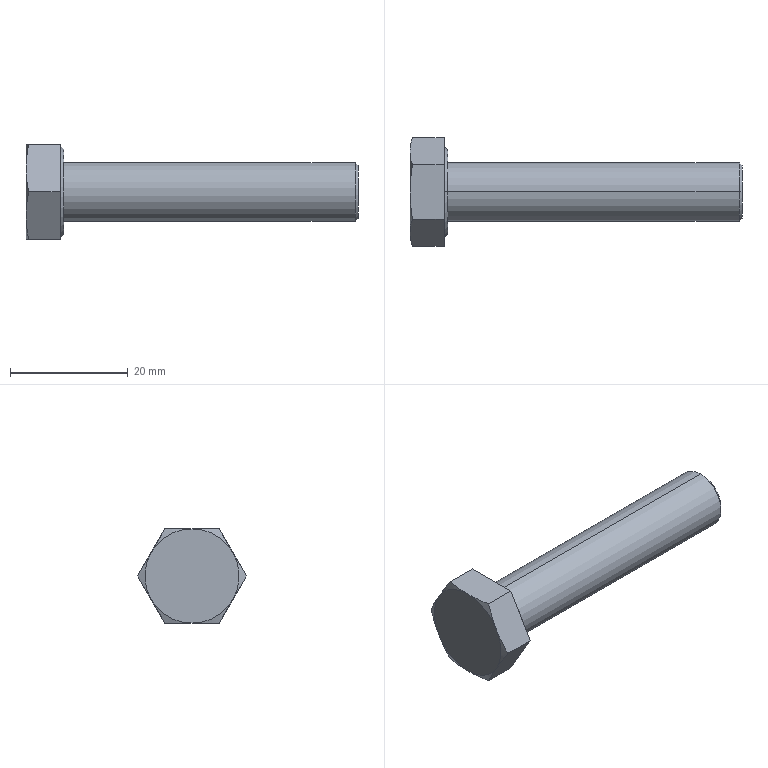Part | SolidWorks | features RevCut 3, Boss 1, Chamfer 1, Extrusion 1, Fillet 1, LPattern 1 | 1 solid | 22 faces | box 56.4 x 18.475 x 16 mm | volume 5313 mm3 | cone 10 | plane 10 | cylinder 2 | commonest cylinder face diameters 10 x2
STEP:
#1=CARTESIAN_POINT('',(56.4,0.,-4.5));
#2=VERTEX_POINT('',#1);
#3=CARTESIAN_POINT('',(56.4,0.,4.5));
#4=VERTEX_POINT('',#3);
#5=CARTESIAN_POINT('',(56.4,0.,0.));
#6=DIRECTION('',(1.,0.,0.));
#7=DIRECTION('',(0.,0.,-1.));
#8=AXIS2_PLACEMENT_3D('',#5,#6,#7);
#9=CIRCLE('',#8,4.5);
#10=EDGE_CURVE('',#2,#4,#9,.T.);
#11=ORIENTED_EDGE('',*,*,#10,.F.);
#12=CARTESIAN_POINT('',(55.9,0.,-5.));
#13=VERTEX_POINT('',#12);
#14=CARTESIAN_POINT('',(56.4,0.,-4.5));
#15=DIRECTION('',(-0.7071,0.,-0.7071));
#16=VECTOR('',#15,1000.);
#17=LINE('',#14,#16);
#18=EDGE_CURVE('',#2,#13,#17,.T.);
#19=ORIENTED_EDGE('',*,*,#18,.T.);
#20=CARTESIAN_POINT('',(55.9,0.,5.));
#21=VERTEX_POINT('',#20);
#22=CARTESIAN_POINT('',(55.9,0.,0.));
#23=DIRECTION('',(-1.,0.,0.));
#24=DIRECTION('',(0.,0.,-1.));
#25=AXIS2_PLACEMENT_3D('',#22,#23,#24);
#26=CIRCLE('',#25,5.);
#27=EDGE_CURVE('',#21,#13,#26,.T.);
#28=ORIENTED_EDGE('',*,*,#27,.F.);
#29=CARTESIAN_POINT('',(56.4,0.,4.5));
#30=DIRECTION('',(-0.7071,0.,0.7071));
#31=VECTOR('',#30,1000.);
#32=LINE('',#29,#31);
#33=EDGE_CURVE('',#4,#21,#32,.T.);
#34=ORIENTED_EDGE('',*,*,#33,.F.);
#35=EDGE_LOOP('',(#11,#19,#28,#34));
#36=FACE_OUTER_BOUND('',#35,.T.);
#37=CARTESIAN_POINT('',(56.4,0.,0.));
#38=DIRECTION('',(-1.,0.,0.));
#39=DIRECTION('',(0.,0.,1.));
#40=AXIS2_PLACEMENT_3D('',#37,#38,#39);
#41=CONICAL_SURFACE('',#40,4.5,0.7854);
#42=ADVANCED_FACE('',(#36),#41,.T.);
#43=ORIENTED_EDGE('',*,*,#27,.T.);
#44=CARTESIAN_POINT('',(6.4,0.,-5.));
#45=VERTEX_POINT('',#44);
#46=CARTESIAN_POINT('',(56.4,0.,-5.));
#47=DIRECTION('',(-1.,0.,0.));
#48=VECTOR('',#47,1000.);
#49=LINE('',#46,#48);
#50=EDGE_CURVE('',#13,#45,#49,.T.);
#51=ORIENTED_EDGE('',*,*,#50,.T.);
#52=CARTESIAN_POINT('',(6.4,0.,5.));
#53=VERTEX_POINT('',#52);
#54=CARTESIAN_POINT('',(6.4,0.,0.));
#55=DIRECTION('',(1.,0.,0.));
#56=DIRECTION('',(0.,0.,-1.));
#57=AXIS2_PLACEMENT_3D('',#54,#55,#56);
#58=CIRCLE('',#57,5.);
#59=EDGE_CURVE('',#45,#53,#58,.T.);
#60=ORIENTED_EDGE('',*,*,#59,.T.);
#61=CARTESIAN_POINT('',(56.4,0.,5.));
#62=DIRECTION('',(-1.,0.,0.));
#63=VECTOR('',#62,1000.);
#64=LINE('',#61,#63);
#65=EDGE_CURVE('',#21,#53,#64,.T.);
#66=ORIENTED_EDGE('',*,*,#65,.F.);
#67=EDGE_LOOP('',(#43,#51,#60,#66));
#68=FACE_OUTER_BOUND('',#67,.T.);
#69=CARTESIAN_POINT('',(56.4,0.,0.));
#70=DIRECTION('',(-1.,0.,0.));
#71=DIRECTION('',(0.,0.,1.));
#72=AXIS2_PLACEMENT_3D('',#69,#70,#71);
#73=CYLINDRICAL_SURFACE('',#72,5.);
#74=ADVANCED_FACE('',(#68),#73,.T.);
#75=CARTESIAN_POINT('',(6.4,0.,7.235));
#76=VERTEX_POINT('',#75);
#77=CARTESIAN_POINT('',(6.4,0.,-7.235));
#78=VERTEX_POINT('',#77);
#79=CARTESIAN_POINT('',(6.4,0.,0.));
#80=DIRECTION('',(-1.,0.,0.));
#81=DIRECTION('',(0.,0.,1.));
#82=AXIS2_PLACEMENT_3D('',#79,#80,#81);
#83=CIRCLE('',#82,7.235);
#84=EDGE_CURVE('',#76,#78,#83,.T.);
#85=ORIENTED_EDGE('',*,*,#84,.T.);
#86=CARTESIAN_POINT('',(5.8,0.,-7.835));
#87=VERTEX_POINT('',#86);
#88=CARTESIAN_POINT('',(5.8,0.,-7.835));
#89=DIRECTION('',(-0.7071,0.,-0.7071));
#90=VECTOR('',#89,1000.);
#91=LINE('',#88,#90);
#92=EDGE_CURVE('',#78,#87,#91,.T.);
#93=ORIENTED_EDGE('',*,*,#92,.T.);
#94=CARTESIAN_POINT('',(5.8,0.,7.835));
#95=VERTEX_POINT('',#94);
#96=CARTESIAN_POINT('',(5.8,0.,0.));
#97=DIRECTION('',(-1.,0.,0.));
#98=DIRECTION('',(0.,0.,1.));
#99=AXIS2_PLACEMENT_3D('',#96,#97,#98);
#100=CIRCLE('',#99,7.835);
#101=EDGE_CURVE('',#95,#87,#100,.T.);
#102=ORIENTED_EDGE('',*,*,#101,.F.);
#103=CARTESIAN_POINT('',(5.8,0.,7.835));
#104=DIRECTION('',(-0.7071,0.,0.7071));
#105=VECTOR('',#104,1000.);
#106=LINE('',#103,#105);
#107=EDGE_CURVE('',#76,#95,#106,.T.);
#108=ORIENTED_EDGE('',*,*,#107,.F.);
#109=EDGE_LOOP('',(#85,#93,#102,#108));
#110=FACE_OUTER_BOUND('',#109,.T.);
#111=CARTESIAN_POINT('',(5.8,0.,0.));
#112=DIRECTION('',(-1.,0.,0.));
#113=DIRECTION('',(0.,0.,1.));
#114=AXIS2_PLACEMENT_3D('',#111,#112,#113);
#115=CONICAL_SURFACE('',#114,7.835,0.7854);
#116=ADVANCED_FACE('',(#110),#115,.T.);
#117=ORIENTED_EDGE('',*,*,#84,.F.);
#118=CARTESIAN_POINT('',(6.4,0.,0.));
#119=DIRECTION('',(-1.,0.,0.));
#120=DIRECTION('',(0.,0.,1.));
#121=AXIS2_PLACEMENT_3D('',#118,#119,#120);
#122=CIRCLE('',#121,7.235);
#123=EDGE_CURVE('',#78,#76,#122,.T.);
#124=ORIENTED_EDGE('',*,*,#123,.F.);
#125=EDGE_LOOP('',(#117,#124));
#126=FACE_OUTER_BOUND('',#125,.T.);
#127=CARTESIAN_POINT('',(6.4,0.,0.));
#128=DIRECTION('',(1.,0.,0.));
#129=DIRECTION('',(0.,0.,-1.));
#130=AXIS2_PLACEMENT_3D('',#127,#128,#129);
#131=CIRCLE('',#130,5.);
#132=EDGE_CURVE('',#53,#45,#131,.T.);
#133=ORIENTED_EDGE('',*,*,#132,.F.);
#134=ORIENTED_EDGE('',*,*,#59,.F.);
#135=EDGE_LOOP('',(#133,#134));
#136=FACE_BOUND('',#135,.T.);
#137=CARTESIAN_POINT('',(6.4,-13.856,-8.));
#138=DIRECTION('',(1.,0.,0.));
#139=DIRECTION('',(0.,0.,-1.));
#140=AXIS2_PLACEMENT_3D('',#137,#138,#139);
#141=PLANE('',#140);
#142=ADVANCED_FACE('',(#126,#136),#141,.T.);
#143=CARTESIAN_POINT('',(0.4505,-9.238,0.));
#144=VERTEX_POINT('',#143);
#145=CARTESIAN_POINT('',(0.,-6.928,4.));
#146=VERTEX_POINT('',#145);
#147=CARTESIAN_POINT('',(0.4505,-9.238,0.));
#148=CARTESIAN_POINT('',(0.3104,-8.853,0.6667));
#149=CARTESIAN_POINT('',(0.1966,-8.468,1.333));
#150=CARTESIAN_POINT('',(0.04119,-7.698,2.667));
#151=CARTESIAN_POINT('',(0.,-7.313,3.333));
#152=CARTESIAN_POINT('',(0.,-6.928,4.));
#153=B_SPLINE_CURVE_WITH_KNOTS('',3,(#147,#148,#149,#150,#151,#152),.UNSPECIFIED.,.F.,.F.,(4,2,4),(0.000000231,0.00231,0.004619),.UNSPECIFIED.);
#154=EDGE_CURVE('',#144,#146,#153,.T.);
#155=ORIENTED_EDGE('',*,*,#154,.F.);
#156=CARTESIAN_POINT('',(5.8,-9.238,0.));
#157=VERTEX_POINT('',#156);
#158=CARTESIAN_POINT('',(6.4,-9.238,0.));
#159=DIRECTION('',(-1.,0.,0.));
#160=VECTOR('',#159,1000.);
#161=LINE('',#158,#160);
#162=EDGE_CURVE('',#157,#144,#161,.T.);
#163=ORIENTED_EDGE('',*,*,#162,.F.);
#164=CARTESIAN_POINT('',(5.8,-4.619,8.));
#165=VERTEX_POINT('',#164);
#166=CARTESIAN_POINT('',(5.8,-4.619,8.));
#167=DIRECTION('',(0.,-0.5,-0.866));
#168=VECTOR('',#167,1000.);
#169=LINE('',#166,#168);
#170=EDGE_CURVE('',#165,#157,#169,.T.);
#171=ORIENTED_EDGE('',*,*,#170,.F.);
#172=CARTESIAN_POINT('',(0.4505,-4.619,8.));
#173=VERTEX_POINT('',#172);
#174=CARTESIAN_POINT('',(6.4,-4.619,8.));
#175=DIRECTION('',(-1.,0.,0.));
#176=VECTOR('',#175,1000.);
#177=LINE('',#174,#176);
#178=EDGE_CURVE('',#165,#173,#177,.T.);
#179=ORIENTED_EDGE('',*,*,#178,.T.);
#180=CARTESIAN_POINT('',(0.,-6.928,4.));
#181=CARTESIAN_POINT('',(0.,-6.543,4.667));
#182=CARTESIAN_POINT('',(0.04119,-6.158,5.333));
#183=CARTESIAN_POINT('',(0.1966,-5.389,6.667));
#184=CARTESIAN_POINT('',(0.3104,-5.004,7.333));
#185=CARTESIAN_POINT('',(0.4505,-4.619,8.));
#186=B_SPLINE_CURVE_WITH_KNOTS('',3,(#180,#181,#182,#183,#184,#185),.UNSPECIFIED.,.F.,.F.,(4,2,4),(0.004619,0.006928,0.009238),.UNSPECIFIED.);
#187=EDGE_CURVE('',#146,#173,#186,.T.);
#188=ORIENTED_EDGE('',*,*,#187,.F.);
#189=EDGE_LOOP('',(#155,#163,#171,#179,#188));
#190=FACE_OUTER_BOUND('',#189,.T.);
#191=CARTESIAN_POINT('',(6.4,-4.619,8.));
#192=DIRECTION('',(0.,0.866,-0.5));
#193=DIRECTION('',(0.,0.5,0.866));
#194=AXIS2_PLACEMENT_3D('',#191,#192,#193);
#195=PLANE('',#194);
#196=ADVANCED_FACE('',(#190),#195,.F.);
#197=CARTESIAN_POINT('',(0.4505,-4.619,-8.));
#198=VERTEX_POINT('',#197);
#199=CARTESIAN_POINT('',(0.,-6.928,-4.));
#200=VERTEX_POINT('',#199);
#201=CARTESIAN_POINT('',(0.4505,-4.619,-8.));
#202=CARTESIAN_POINT('',(0.3104,-5.004,-7.333));
#203=CARTESIAN_POINT('',(0.1966,-5.389,-6.667));
#204=CARTESIAN_POINT('',(0.04119,-6.158,-5.333));
#205=CARTESIAN_POINT('',(0.,-6.543,-4.667));
#206=CARTESIAN_POINT('',(0.,-6.928,-4.));
#207=B_SPLINE_CURVE_WITH_KNOTS('',3,(#201,#202,#203,#204,#205,#206),.UNSPECIFIED.,.F.,.F.,(4,2,4),(0.000000231,0.00231,0.004619),.UNSPECIFIED.);
#208=EDGE_CURVE('',#198,#200,#207,.T.);
#209=ORIENTED_EDGE('',*,*,#208,.F.);
#210=CARTESIAN_POINT('',(5.8,-4.619,-8.));
#211=VERTEX_POINT('',#210);
#212=CARTESIAN_POINT('',(6.4,-4.619,-8.));
#213=DIRECTION('',(-1.,0.,0.));
#214=VECTOR('',#213,1000.);
#215=LINE('',#212,#214);
#216=EDGE_CURVE('',#211,#198,#215,.T.);
#217=ORIENTED_EDGE('',*,*,#216,.F.);
#218=CARTESIAN_POINT('',(5.8,-9.238,0.));
#219=DIRECTION('',(0.,0.5,-0.866));
#220=VECTOR('',#219,1000.);
#221=LINE('',#218,#220);
#222=EDGE_CURVE('',#157,#211,#221,.T.);
#223=ORIENTED_EDGE('',*,*,#222,.F.);
#224=ORIENTED_EDGE('',*,*,#162,.T.);
#225=CARTESIAN_POINT('',(0.,-6.928,-4.));
#226=CARTESIAN_POINT('',(0.,-7.313,-3.333));
#227=CARTESIAN_POINT('',(0.04119,-7.698,-2.667));
#228=CARTESIAN_POINT('',(0.1966,-8.468,-1.333));
#229=CARTESIAN_POINT('',(0.3104,-8.853,-0.6667));
#230=CARTESIAN_POINT('',(0.4505,-9.238,0.));
#231=B_SPLINE_CURVE_WITH_KNOTS('',3,(#225,#226,#227,#228,#229,#230),.UNSPECIFIED.,.F.,.F.,(4,2,4),(0.004619,0.006928,0.009238),.UNSPECIFIED.);
#232=EDGE_CURVE('',#200,#144,#231,.T.);
#233=ORIENTED_EDGE('',*,*,#232,.F.);
#234=EDGE_LOOP('',(#209,#217,#223,#224,#233));
#235=FACE_OUTER_BOUND('',#234,.T.);
#236=CARTESIAN_POINT('',(6.4,-9.238,0.));
#237=DIRECTION('',(0.,0.866,0.5));
#238=DIRECTION('',(0.,-0.5,0.866));
#239=AXIS2_PLACEMENT_3D('',#236,#237,#238);
#240=PLANE('',#239);
#241=ADVANCED_FACE('',(#235),#240,.F.);
#242=CARTESIAN_POINT('',(0.4505,4.619,-8.));
#243=VERTEX_POINT('',#242);
#244=CARTESIAN_POINT('',(0.,0.,-8.));
#245=VERTEX_POINT('',#244);
#246=CARTESIAN_POINT('',(0.4505,4.619,-8.));
#247=CARTESIAN_POINT('',(0.3107,3.851,-8.));
#248=CARTESIAN_POINT('',(0.1969,3.081,-8.));
#249=CARTESIAN_POINT('',(0.04135,1.542,-8.));
#250=CARTESIAN_POINT('',(0.,0.7714,-8.));
#251=CARTESIAN_POINT('',(0.,0.,-8.));
#252=B_SPLINE_CURVE_WITH_KNOTS('',3,(#246,#247,#248,#249,#250,#251),.UNSPECIFIED.,.F.,.F.,(4,2,4),(0.01666,0.01898,0.02131),.UNSPECIFIED.);
#253=EDGE_CURVE('',#243,#245,#252,.T.);
#254=ORIENTED_EDGE('',*,*,#253,.F.);
#255=CARTESIAN_POINT('',(5.8,4.619,-8.));
#256=VERTEX_POINT('',#255);
#257=CARTESIAN_POINT('',(6.4,4.619,-8.));
#258=DIRECTION('',(-1.,0.,0.));
#259=VECTOR('',#258,1000.);
#260=LINE('',#257,#259);
#261=EDGE_CURVE('',#256,#243,#260,.T.);
#262=ORIENTED_EDGE('',*,*,#261,.F.);
#263=CARTESIAN_POINT('',(5.8,-4.619,-8.));
#264=DIRECTION('',(0.,1.,0.));
#265=VECTOR('',#264,1000.);
#266=LINE('',#263,#265);
#267=EDGE_CURVE('',#211,#256,#266,.T.);
#268=ORIENTED_EDGE('',*,*,#267,.F.);
#269=ORIENTED_EDGE('',*,*,#216,.T.);
#270=CARTESIAN_POINT('',(0.,0.,-8.));
#271=CARTESIAN_POINT('',(0.,-0.7692,-8.));
#272=CARTESIAN_POINT('',(0.04113,-1.539,-8.));
#273=CARTESIAN_POINT('',(0.1968,-3.081,-8.));
#274=CARTESIAN_POINT('',(0.3113,-3.854,-8.));
#275=CARTESIAN_POINT('',(0.4505,-4.619,-8.));
#276=B_SPLINE_CURVE_WITH_KNOTS('',3,(#270,#271,#272,#273,#274,#275),.UNSPECIFIED.,.F.,.F.,(4,2,4),(0.02131,0.02363,0.02596),.UNSPECIFIED.);
#277=EDGE_CURVE('',#245,#198,#276,.T.);
#278=ORIENTED_EDGE('',*,*,#277,.F.);
#279=EDGE_LOOP('',(#254,#262,#268,#269,#278));
#280=FACE_OUTER_BOUND('',#279,.T.);
#281=CARTESIAN_POINT('',(6.4,-4.619,-8.));
#282=DIRECTION('',(0.,0.,1.));
#283=DIRECTION('',(1.,0.,0.));
#284=AXIS2_PLACEMENT_3D('',#281,#282,#283);
#285=PLANE('',#284);
#286=ADVANCED_FACE('',(#280),#285,.F.);
#287=CARTESIAN_POINT('',(0.4505,9.238,0.));
#288=VERTEX_POINT('',#287);
#289=CARTESIAN_POINT('',(0.,6.928,-4.));
#290=VERTEX_POINT('',#289);
#291=CARTESIAN_POINT('',(0.4505,9.238,0.));
#292=CARTESIAN_POINT('',(0.3104,8.853,-0.6667));
#293=CARTESIAN_POINT('',(0.1966,8.468,-1.333));
#294=CARTESIAN_POINT('',(0.04119,7.698,-2.667));
#295=CARTESIAN_POINT('',(0.,7.313,-3.333));
#296=CARTESIAN_POINT('',(0.,6.928,-4.));
#297=B_SPLINE_CURVE_WITH_KNOTS('',3,(#291,#292,#293,#294,#295,#296),.UNSPECIFIED.,.F.,.F.,(4,2,4),(0.000000231,0.00231,0.004619),.UNSPECIFIED.);
#298=EDGE_CURVE('',#288,#290,#297,.T.);
#299=ORIENTED_EDGE('',*,*,#298,.F.);
#300=CARTESIAN_POINT('',(5.8,9.238,0.));
#301=VERTEX_POINT('',#300);
#302=CARTESIAN_POINT('',(6.4,9.238,0.));
#303=DIRECTION('',(-1.,0.,0.));
#304=VECTOR('',#303,1000.);
#305=LINE('',#302,#304);
#306=EDGE_CURVE('',#301,#288,#305,.T.);
#307=ORIENTED_EDGE('',*,*,#306,.F.);
#308=CARTESIAN_POINT('',(5.8,4.619,-8.));
#309=DIRECTION('',(0.,0.5,0.866));
#310=VECTOR('',#309,1000.);
#311=LINE('',#308,#310);
#312=EDGE_CURVE('',#256,#301,#311,.T.);
#313=ORIENTED_EDGE('',*,*,#312,.F.);
#314=ORIENTED_EDGE('',*,*,#261,.T.);
#315=CARTESIAN_POINT('',(0.,6.928,-4.));
#316=CARTESIAN_POINT('',(0.,6.543,-4.667));
#317=CARTESIAN_POINT('',(0.04119,6.158,-5.333));
#318=CARTESIAN_POINT('',(0.1966,5.389,-6.667));
#319=CARTESIAN_POINT('',(0.3104,5.004,-7.333));
#320=CARTESIAN_POINT('',(0.4505,4.619,-8.));
#321=B_SPLINE_CURVE_WITH_KNOTS('',3,(#315,#316,#317,#318,#319,#320),.UNSPECIFIED.,.F.,.F.,(4,2,4),(0.004619,0.006928,0.009238),.UNSPECIFIED.);
#322=EDGE_CURVE('',#290,#243,#321,.T.);
#323=ORIENTED_EDGE('',*,*,#322,.F.);
#324=EDGE_LOOP('',(#299,#307,#313,#314,#323));
#325=FACE_OUTER_BOUND('',#324,.T.);
#326=CARTESIAN_POINT('',(6.4,4.619,-8.));
#327=DIRECTION('',(0.,-0.866,0.5));
#328=DIRECTION('',(0.,-0.5,-0.866));
#329=AXIS2_PLACEMENT_3D('',#326,#327,#328);
#330=PLANE('',#329);
#331=ADVANCED_FACE('',(#325),#330,.F.);
#332=CARTESIAN_POINT('',(0.4505,4.619,8.));
#333=VERTEX_POINT('',#332);
#334=CARTESIAN_POINT('',(0.,6.928,4.));
#335=VERTEX_POINT('',#334);
#336=CARTESIAN_POINT('',(0.4505,4.619,8.));
#337=CARTESIAN_POINT('',(0.3104,5.004,7.333));
#338=CARTESIAN_POINT('',(0.1966,5.389,6.667));
#339=CARTESIAN_POINT('',(0.04119,6.158,5.333));
#340=CARTESIAN_POINT('',(0.,6.543,4.667));
#341=CARTESIAN_POINT('',(0.,6.928,4.));
#342=B_SPLINE_CURVE_WITH_KNOTS('',3,(#336,#337,#338,#339,#340,#341),.UNSPECIFIED.,.F.,.F.,(4,2,4),(0.000000231,0.00231,0.004619),.UNSPECIFIED.);
#343=EDGE_CURVE('',#333,#335,#342,.T.);
#344=ORIENTED_EDGE('',*,*,#343,.F.);
#345=CARTESIAN_POINT('',(5.8,4.619,8.));
#346=VERTEX_POINT('',#345);
#347=CARTESIAN_POINT('',(6.4,4.619,8.));
#348=DIRECTION('',(-1.,0.,0.));
#349=VECTOR('',#348,1000.);
#350=LINE('',#347,#349);
#351=EDGE_CURVE('',#346,#333,#350,.T.);
#352=ORIENTED_EDGE('',*,*,#351,.F.);
#353=CARTESIAN_POINT('',(5.8,9.238,0.));
#354=DIRECTION('',(0.,-0.5,0.866));
#355=VECTOR('',#354,1000.);
#356=LINE('',#353,#355);
#357=EDGE_CURVE('',#301,#346,#356,.T.);
#358=ORIENTED_EDGE('',*,*,#357,.F.);
#359=ORIENTED_EDGE('',*,*,#306,.T.);
#360=CARTESIAN_POINT('',(0.,6.928,4.));
#361=CARTESIAN_POINT('',(0.,7.313,3.333));
#362=CARTESIAN_POINT('',(0.04119,7.698,2.667));
#363=CARTESIAN_POINT('',(0.1966,8.468,1.333));
#364=CARTESIAN_POINT('',(0.3104,8.853,0.6667));
#365=CARTESIAN_POINT('',(0.4505,9.238,0.));
#366=B_SPLINE_CURVE_WITH_KNOTS('',3,(#360,#361,#362,#363,#364,#365),.UNSPECIFIED.,.F.,.F.,(4,2,4),(0.004619,0.006928,0.009238),.UNSPECIFIED.);
#367=EDGE_CURVE('',#335,#288,#366,.T.);
#368=ORIENTED_EDGE('',*,*,#367,.F.);
#369=EDGE_LOOP('',(#344,#352,#358,#359,#368));
#370=FACE_OUTER_BOUND('',#369,.T.);
#371=CARTESIAN_POINT('',(6.4,9.238,0.));
#372=DIRECTION('',(0.,-0.866,-0.5));
#373=DIRECTION('',(0.,0.5,-0.866));
#374=AXIS2_PLACEMENT_3D('',#371,#372,#373);
#375=PLANE('',#374);
#376=ADVANCED_FACE('',(#370),#375,.F.);
#377=CARTESIAN_POINT('',(0.,0.,8.));
#378=VERTEX_POINT('',#377);
#379=CARTESIAN_POINT('',(0.4505,-4.619,8.));
#380=CARTESIAN_POINT('',(0.3113,-3.854,8.));
#381=CARTESIAN_POINT('',(0.1968,-3.081,8.));
#382=CARTESIAN_POINT('',(0.04113,-1.539,8.));
#383=CARTESIAN_POINT('',(0.,-0.7692,8.));
#384=CARTESIAN_POINT('',(0.,0.,8.));
#385=B_SPLINE_CURVE_WITH_KNOTS('',3,(#379,#380,#381,#382,#383,#384),.UNSPECIFIED.,.F.,.F.,(4,2,4),(0.007857,0.01018,0.01251),.UNSPECIFIED.);
#386=EDGE_CURVE('',#173,#378,#385,.T.);
#387=ORIENTED_EDGE('',*,*,#386,.F.);
#388=ORIENTED_EDGE('',*,*,#178,.F.);
#389=CARTESIAN_POINT('',(5.8,4.619,8.));
#390=DIRECTION('',(0.,-1.,0.));
#391=VECTOR('',#390,1000.);
#392=LINE('',#389,#391);
#393=EDGE_CURVE('',#346,#165,#392,.T.);
#394=ORIENTED_EDGE('',*,*,#393,.F.);
#395=ORIENTED_EDGE('',*,*,#351,.T.);
#396=CARTESIAN_POINT('',(0.,0.,8.));
#397=CARTESIAN_POINT('',(0.,0.7714,8.));
#398=CARTESIAN_POINT('',(0.04135,1.542,8.));
#399=CARTESIAN_POINT('',(0.1969,3.081,8.));
#400=CARTESIAN_POINT('',(0.3107,3.851,8.));
#401=CARTESIAN_POINT('',(0.4505,4.619,8.));
#402=B_SPLINE_CURVE_WITH_KNOTS('',3,(#396,#397,#398,#399,#400,#401),.UNSPECIFIED.,.F.,.F.,(4,2,4),(0.01251,0.01485,0.01718),.UNSPECIFIED.);
#403=EDGE_CURVE('',#378,#333,#402,.T.);
#404=ORIENTED_EDGE('',*,*,#403,.F.);
#405=EDGE_LOOP('',(#387,#388,#394,#395,#404));
#406=FACE_OUTER_BOUND('',#405,.T.);
#407=CARTESIAN_POINT('',(6.4,4.619,8.));
#408=DIRECTION('',(0.,0.,-1.));
#409=DIRECTION('',(0.,1.,0.));
#410=AXIS2_PLACEMENT_3D('',#407,#408,#409);
#411=PLANE('',#410);
#412=ADVANCED_FACE('',(#406),#411,.F.);
#413=ORIENTED_EDGE('',*,*,#101,.T.);
#414=CARTESIAN_POINT('',(5.8,0.,0.));
#415=DIRECTION('',(-1.,0.,0.));
#416=DIRECTION('',(0.,0.,1.));
#417=AXIS2_PLACEMENT_3D('',#414,#415,#416);
#418=CIRCLE('',#417,7.835);
#419=EDGE_CURVE('',#87,#95,#418,.T.);
#420=ORIENTED_EDGE('',*,*,#419,.T.);
#421=EDGE_LOOP('',(#413,#420));
#422=FACE_BOUND('',#421,.T.);
#423=ORIENTED_EDGE('',*,*,#170,.T.);
#424=ORIENTED_EDGE('',*,*,#222,.T.);
#425=ORIENTED_EDGE('',*,*,#267,.T.);
#426=ORIENTED_EDGE('',*,*,#312,.T.);
#427=ORIENTED_EDGE('',*,*,#357,.T.);
#428=ORIENTED_EDGE('',*,*,#393,.T.);
#429=EDGE_LOOP('',(#423,#424,#425,#426,#427,#428));
#430=FACE_OUTER_BOUND('',#429,.T.);
#431=CARTESIAN_POINT('',(5.8,7.835,0.));
#432=DIRECTION('',(1.,0.,0.));
#433=DIRECTION('',(0.,0.,-1.));
#434=AXIS2_PLACEMENT_3D('',#431,#432,#433);
#435=PLANE('',#434);
#436=ADVANCED_FACE('',(#422,#430),#435,.T.);
#437=ORIENTED_EDGE('',*,*,#92,.F.);
#438=ORIENTED_EDGE('',*,*,#123,.T.);
#439=ORIENTED_EDGE('',*,*,#107,.T.);
#440=ORIENTED_EDGE('',*,*,#419,.F.);
#441=EDGE_LOOP('',(#437,#438,#439,#440));
#442=FACE_OUTER_BOUND('',#441,.T.);
#443=CARTESIAN_POINT('',(5.8,0.,0.));
#444=DIRECTION('',(-1.,0.,0.));
#445=DIRECTION('',(0.,0.,1.));
#446=AXIS2_PLACEMENT_3D('',#443,#444,#445);
#447=CONICAL_SURFACE('',#446,7.835,0.7854);
#448=ADVANCED_FACE('',(#442),#447,.T.);
#449=ORIENTED_EDGE('',*,*,#277,.T.);
#450=ORIENTED_EDGE('',*,*,#208,.T.);
#451=CARTESIAN_POINT('',(0.,0.,0.));
#452=DIRECTION('',(1.,0.,0.));
#453=DIRECTION('',(0.,0.,-1.));
#454=AXIS2_PLACEMENT_3D('',#451,#452,#453);
#455=CIRCLE('',#454,8.);
#456=EDGE_CURVE('',#200,#245,#455,.T.);
#457=ORIENTED_EDGE('',*,*,#456,.T.);
#458=EDGE_LOOP('',(#449,#450,#457));
#459=FACE_OUTER_BOUND('',#458,.T.);
#460=CARTESIAN_POINT('',(0.,0.,0.));
#461=DIRECTION('',(1.,0.,0.));
#462=DIRECTION('',(0.,0.,-1.));
#463=AXIS2_PLACEMENT_3D('',#460,#461,#462);
#464=CONICAL_SURFACE('',#463,8.,1.222);
#465=ADVANCED_FACE('',(#459),#464,.T.);
#466=ORIENTED_EDGE('',*,*,#232,.T.);
#467=ORIENTED_EDGE('',*,*,#154,.T.);
#468=CARTESIAN_POINT('',(0.,0.,0.));
#469=DIRECTION('',(1.,0.,0.));
#470=DIRECTION('',(0.,0.,-1.));
#471=AXIS2_PLACEMENT_3D('',#468,#469,#470);
#472=CIRCLE('',#471,8.);
#473=EDGE_CURVE('',#146,#200,#472,.T.);
#474=ORIENTED_EDGE('',*,*,#473,.T.);
#475=EDGE_LOOP('',(#466,#467,#474));
#476=FACE_OUTER_BOUND('',#475,.T.);
#477=CARTESIAN_POINT('',(0.,0.,0.));
#478=DIRECTION('',(1.,0.,0.));
#479=DIRECTION('',(0.,0.,-1.));
#480=AXIS2_PLACEMENT_3D('',#477,#478,#479);
#481=CONICAL_SURFACE('',#480,8.,1.222);
#482=ADVANCED_FACE('',(#476),#481,.T.);
#483=ORIENTED_EDGE('',*,*,#187,.T.);
#484=ORIENTED_EDGE('',*,*,#386,.T.);
#485=CARTESIAN_POINT('',(0.,0.,0.));
#486=DIRECTION('',(1.,0.,0.));
#487=DIRECTION('',(0.,0.,-1.));
#488=AXIS2_PLACEMENT_3D('',#485,#486,#487);
#489=CIRCLE('',#488,8.);
#490=EDGE_CURVE('',#378,#146,#489,.T.);
#491=ORIENTED_EDGE('',*,*,#490,.T.);
#492=EDGE_LOOP('',(#483,#484,#491));
#493=FACE_OUTER_BOUND('',#492,.T.);
#494=CARTESIAN_POINT('',(0.,0.,0.));
#495=DIRECTION('',(1.,0.,0.));
#496=DIRECTION('',(0.,0.,-1.));
#497=AXIS2_PLACEMENT_3D('',#494,#495,#496);
#498=CONICAL_SURFACE('',#497,8.,1.222);
#499=ADVANCED_FACE('',(#493),#498,.T.);
#500=ORIENTED_EDGE('',*,*,#343,.T.);
#501=CARTESIAN_POINT('',(0.,0.,0.));
#502=DIRECTION('',(-1.,0.,0.));
#503=DIRECTION('',(0.,0.,1.));
#504=AXIS2_PLACEMENT_3D('',#501,#502,#503);
#505=CIRCLE('',#504,8.);
#506=EDGE_CURVE('',#378,#335,#505,.T.);
#507=ORIENTED_EDGE('',*,*,#506,.F.);
#508=ORIENTED_EDGE('',*,*,#403,.T.);
#509=EDGE_LOOP('',(#500,#507,#508));
#510=FACE_OUTER_BOUND('',#509,.T.);
#511=CARTESIAN_POINT('',(0.,0.,0.));
#512=DIRECTION('',(1.,0.,0.));
#513=DIRECTION('',(0.,0.,-1.));
#514=AXIS2_PLACEMENT_3D('',#511,#512,#513);
#515=CONICAL_SURFACE('',#514,8.,1.222);
#516=ADVANCED_FACE('',(#510),#515,.T.);
#517=ORIENTED_EDGE('',*,*,#298,.T.);
#518=CARTESIAN_POINT('',(0.,0.,0.));
#519=DIRECTION('',(1.,0.,0.));
#520=DIRECTION('',(0.,0.,-1.));
#521=AXIS2_PLACEMENT_3D('',#518,#519,#520);
#522=CIRCLE('',#521,8.);
#523=EDGE_CURVE('',#290,#335,#522,.T.);
#524=ORIENTED_EDGE('',*,*,#523,.T.);
#525=ORIENTED_EDGE('',*,*,#367,.T.);
#526=EDGE_LOOP('',(#517,#524,#525));
#527=FACE_OUTER_BOUND('',#526,.T.);
#528=CARTESIAN_POINT('',(0.,0.,0.));
#529=DIRECTION('',(1.,0.,0.));
#530=DIRECTION('',(0.,0.,-1.));
#531=AXIS2_PLACEMENT_3D('',#528,#529,#530);
#532=CONICAL_SURFACE('',#531,8.,1.222);
#533=ADVANCED_FACE('',(#527),#532,.T.);
#534=ORIENTED_EDGE('',*,*,#253,.T.);
#535=CARTESIAN_POINT('',(0.,0.,0.));
#536=DIRECTION('',(1.,0.,0.));
#537=DIRECTION('',(0.,0.,-1.));
#538=AXIS2_PLACEMENT_3D('',#535,#536,#537);
#539=CIRCLE('',#538,8.);
#540=EDGE_CURVE('',#245,#290,#539,.T.);
#541=ORIENTED_EDGE('',*,*,#540,.T.);
#542=ORIENTED_EDGE('',*,*,#322,.T.);
#543=EDGE_LOOP('',(#534,#541,#542));
#544=FACE_OUTER_BOUND('',#543,.T.);
#545=CARTESIAN_POINT('',(0.,0.,0.));
#546=DIRECTION('',(1.,0.,0.));
#547=DIRECTION('',(0.,0.,-1.));
#548=AXIS2_PLACEMENT_3D('',#545,#546,#547);
#549=CONICAL_SURFACE('',#548,8.,1.222);
#550=ADVANCED_FACE('',(#544),#549,.T.);
#551=ORIENTED_EDGE('',*,*,#540,.F.);
#552=ORIENTED_EDGE('',*,*,#456,.F.);
#553=ORIENTED_EDGE('',*,*,#473,.F.);
#554=ORIENTED_EDGE('',*,*,#490,.F.);
#555=ORIENTED_EDGE('',*,*,#506,.T.);
#556=ORIENTED_EDGE('',*,*,#523,.F.);
#557=EDGE_LOOP('',(#551,#552,#553,#554,#555,#556));
#558=FACE_OUTER_BOUND('',#557,.T.);
#559=CARTESIAN_POINT('',(0.,-13.856,-8.));
#560=DIRECTION('',(1.,0.,0.));
#561=DIRECTION('',(0.,0.,-1.));
#562=AXIS2_PLACEMENT_3D('',#559,#560,#561);
#563=PLANE('',#562);
#564=ADVANCED_FACE('',(#558),#563,.F.);
#565=ORIENTED_EDGE('',*,*,#50,.F.);
#566=CARTESIAN_POINT('',(55.9,0.,0.));
#567=DIRECTION('',(-1.,0.,0.));
#568=DIRECTION('',(0.,0.,-1.));
#569=AXIS2_PLACEMENT_3D('',#566,#567,#568);
#570=CIRCLE('',#569,5.);
#571=EDGE_CURVE('',#13,#21,#570,.T.);
#572=ORIENTED_EDGE('',*,*,#571,.T.);
#573=ORIENTED_EDGE('',*,*,#65,.T.);
#574=ORIENTED_EDGE('',*,*,#132,.T.);
#575=EDGE_LOOP('',(#565,#572,#573,#574));
#576=FACE_OUTER_BOUND('',#575,.T.);
#577=CARTESIAN_POINT('',(56.4,0.,0.));
#578=DIRECTION('',(-1.,0.,0.));
#579=DIRECTION('',(0.,0.,1.));
#580=AXIS2_PLACEMENT_3D('',#577,#578,#579);
#581=CYLINDRICAL_SURFACE('',#580,5.);
#582=ADVANCED_FACE('',(#576),#581,.T.);
#583=CARTESIAN_POINT('',(56.4,0.,0.));
#584=DIRECTION('',(1.,0.,0.));
#585=DIRECTION('',(0.,0.,-1.));
#586=AXIS2_PLACEMENT_3D('',#583,#584,#585);
#587=CIRCLE('',#586,4.5);
#588=EDGE_CURVE('',#4,#2,#587,.T.);
#589=ORIENTED_EDGE('',*,*,#588,.T.);
#590=ORIENTED_EDGE('',*,*,#10,.T.);
#591=EDGE_LOOP('',(#589,#590));
#592=FACE_OUTER_BOUND('',#591,.T.);
#593=CARTESIAN_POINT('',(56.4,0.,0.));
#594=DIRECTION('',(1.,0.,0.));
#595=DIRECTION('',(0.,0.,-1.));
#596=AXIS2_PLACEMENT_3D('',#593,#594,#595);
#597=PLANE('',#596);
#598=ADVANCED_FACE('',(#592),#597,.T.);
#599=ORIENTED_EDGE('',*,*,#18,.F.);
#600=ORIENTED_EDGE('',*,*,#588,.F.);
#601=ORIENTED_EDGE('',*,*,#33,.T.);
#602=ORIENTED_EDGE('',*,*,#571,.F.);
#603=EDGE_LOOP('',(#599,#600,#601,#602));
#604=FACE_OUTER_BOUND('',#603,.T.);
#605=CARTESIAN_POINT('',(56.4,0.,0.));
#606=DIRECTION('',(-1.,0.,0.));
#607=DIRECTION('',(0.,0.,1.));
#608=AXIS2_PLACEMENT_3D('',#605,#606,#607);
#609=CONICAL_SURFACE('',#608,4.5,0.7854);
#610=ADVANCED_FACE('',(#604),#609,.T.);
#611=CLOSED_SHELL('',(#42,#74,#116,#142,#196,#241,#286,#331,#376,#412,#436,#448,#465,#482,#499,#516,#533,#550,#564,#582,#598,#610));
#612=MANIFOLD_SOLID_BREP('',#611);
#613=CARTESIAN_POINT('',(0.,0.,0.));
#614=DIRECTION('',(0.,0.,1.));
#615=DIRECTION('',(1.,0.,0.));
#616=AXIS2_PLACEMENT_3D('',#613,#614,#615);
#617=(LENGTH_UNIT()NAMED_UNIT(*)SI_UNIT(.MILLI.,.METRE.));
#618=UNCERTAINTY_MEASURE_WITH_UNIT(LENGTH_MEASURE(0.00001),#617,'','');
#619=(NAMED_UNIT(*)PLANE_ANGLE_UNIT()SI_UNIT($,.RADIAN.));
#620=(NAMED_UNIT(*)SI_UNIT($,.STERADIAN.)SOLID_ANGLE_UNIT());
#621=(GEOMETRIC_REPRESENTATION_CONTEXT(3)GLOBAL_UNCERTAINTY_ASSIGNED_CONTEXT((#618))GLOBAL_UNIT_ASSIGNED_CONTEXT((#617,#619,#620))REPRESENTATION_CONTEXT('',''));
#622=ADVANCED_BREP_SHAPE_REPRESENTATION('',(#612,#616),#621);